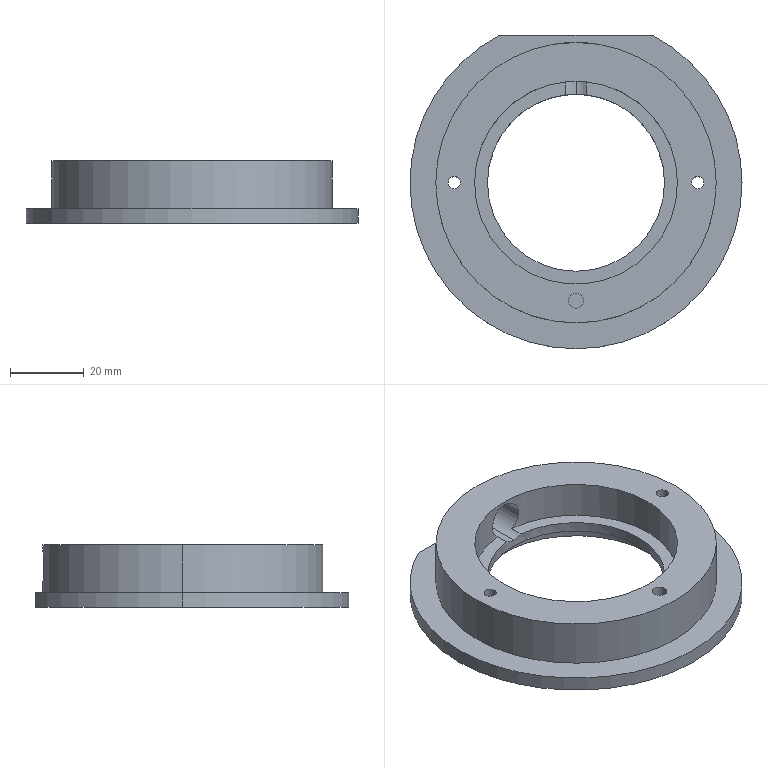Part | STEP file | PN_0096 fixed round plate | 1 solid | 26 faces | box 90 x 85 x 17 mm | volume 43807 mm3 | cylinder 19 | plane 7 | commonest cylinder face diameters 3.3 x4 55 x4 90 x3 4 x2 10 x2 48 x2